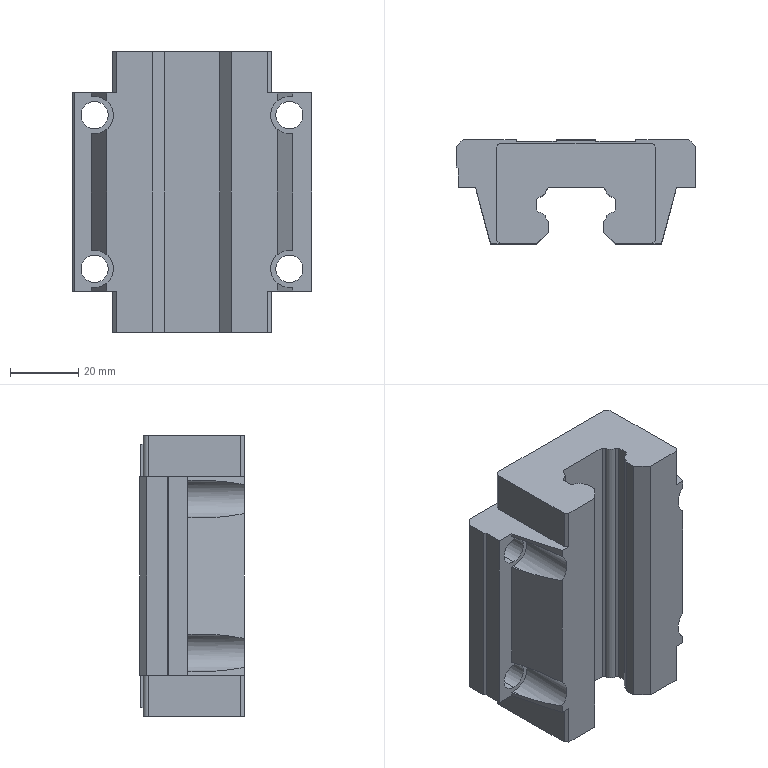Part | SolidWorks | 1 solid | 90 faces | box 70 x 30.5 x 82 mm | volume 109676 mm3 | plane 70 | cylinder 20 | commonest cylinder face diameters 8 x8 3 x4 4.6 x4 11 x4